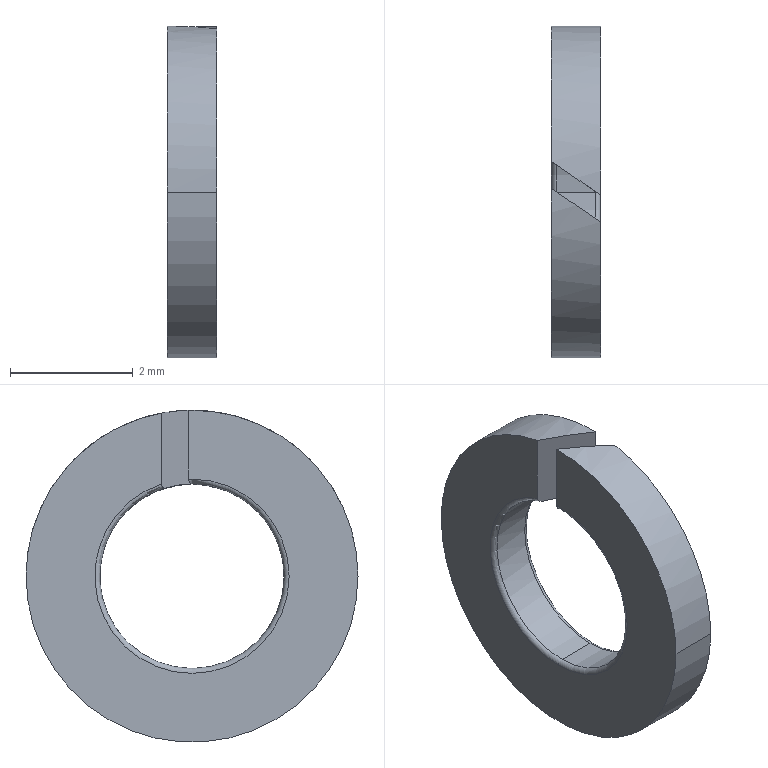Part | STEP file | ASSEMBLY_GB_T_9074_4_M3X8_2 | 1 solid | 11 faces | box 0.8 x 5.4 x 5.4 mm | volume 12.217 mm3 | cylinder 5 | plane 4 | torus 2 | commonest cylinder face diameters 5.4 x3 3 x2